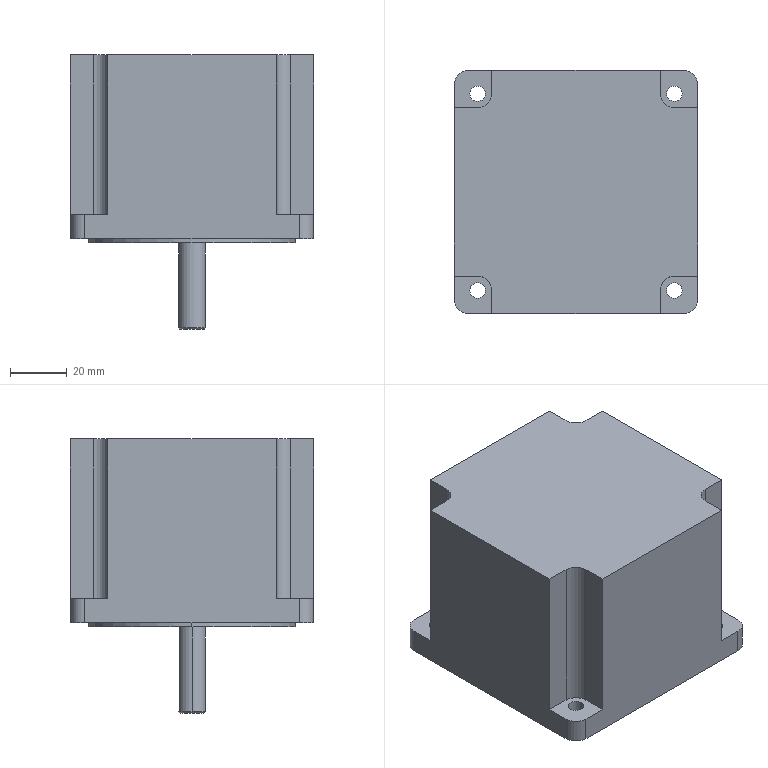Part | STEP file | 86HS35 | 1 solid | 42 faces | box 86 x 86 x 97 mm | volume 450020 mm3 | cylinder 20 | plane 20 | cone 2 | commonest cylinder face diameters 5.5 x8 10 x8 9.5 x2 73 x2